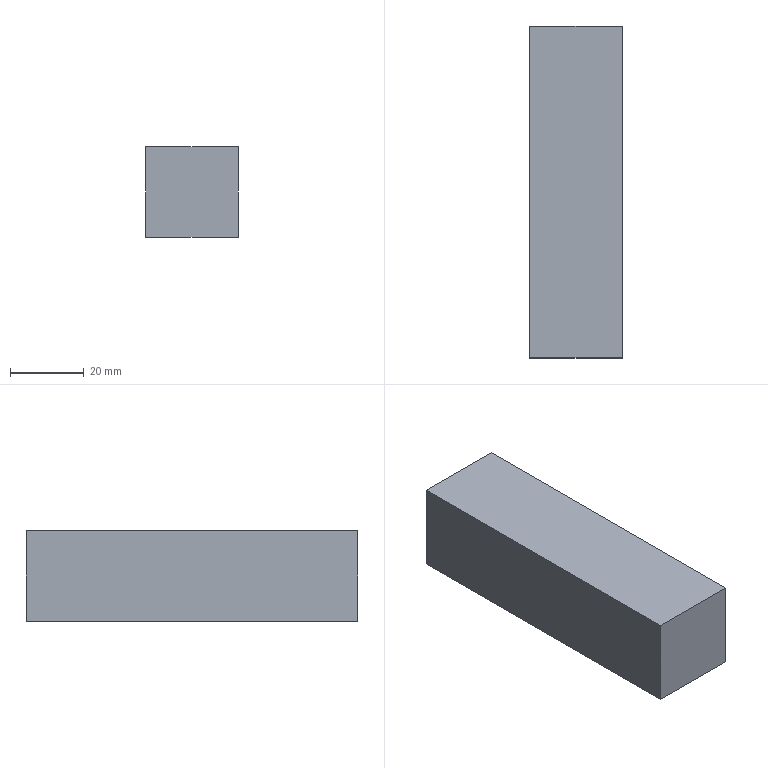Part | SolidWorks | features Extrusion 1 | 1 solid | 6 faces | box 25 x 90 x 24.5 mm | volume 55125 mm3 | plane 6
STEP:
#1=CARTESIAN_POINT('',(0.,45.,0.));
#2=VERTEX_POINT('',#1);
#3=CARTESIAN_POINT('',(0.,-45.,0.));
#4=VERTEX_POINT('',#3);
#5=CARTESIAN_POINT('',(0.,45.,0.));
#6=DIRECTION('',(0.,-1.,0.));
#7=VECTOR('',#6,1000.);
#8=LINE('',#5,#7);
#9=EDGE_CURVE('',#2,#4,#8,.T.);
#10=ORIENTED_EDGE('',*,*,#9,.T.);
#11=CARTESIAN_POINT('',(0.,-45.,24.5));
#12=VERTEX_POINT('',#11);
#13=CARTESIAN_POINT('',(0.,-45.,24.5));
#14=DIRECTION('',(0.,0.,-1.));
#15=VECTOR('',#14,1000.);
#16=LINE('',#13,#15);
#17=EDGE_CURVE('',#12,#4,#16,.T.);
#18=ORIENTED_EDGE('',*,*,#17,.F.);
#19=CARTESIAN_POINT('',(0.,45.,24.5));
#20=VERTEX_POINT('',#19);
#21=CARTESIAN_POINT('',(0.,45.,24.5));
#22=DIRECTION('',(0.,-1.,0.));
#23=VECTOR('',#22,1000.);
#24=LINE('',#21,#23);
#25=EDGE_CURVE('',#20,#12,#24,.T.);
#26=ORIENTED_EDGE('',*,*,#25,.F.);
#27=CARTESIAN_POINT('',(0.,45.,24.5));
#28=DIRECTION('',(0.,0.,-1.));
#29=VECTOR('',#28,1000.);
#30=LINE('',#27,#29);
#31=EDGE_CURVE('',#20,#2,#30,.T.);
#32=ORIENTED_EDGE('',*,*,#31,.T.);
#33=EDGE_LOOP('',(#10,#18,#26,#32));
#34=FACE_OUTER_BOUND('',#33,.T.);
#35=CARTESIAN_POINT('',(0.,45.,24.5));
#36=DIRECTION('',(1.,0.,0.));
#37=DIRECTION('',(0.,0.,-1.));
#38=AXIS2_PLACEMENT_3D('',#35,#36,#37);
#39=PLANE('',#38);
#40=ADVANCED_FACE('',(#34),#39,.F.);
#41=CARTESIAN_POINT('',(25.,-45.,0.));
#42=VERTEX_POINT('',#41);
#43=CARTESIAN_POINT('',(0.,-45.,0.));
#44=DIRECTION('',(1.,0.,0.));
#45=VECTOR('',#44,1000.);
#46=LINE('',#43,#45);
#47=EDGE_CURVE('',#4,#42,#46,.T.);
#48=ORIENTED_EDGE('',*,*,#47,.T.);
#49=CARTESIAN_POINT('',(25.,-45.,24.5));
#50=VERTEX_POINT('',#49);
#51=CARTESIAN_POINT('',(25.,-45.,24.5));
#52=DIRECTION('',(0.,0.,-1.));
#53=VECTOR('',#52,1000.);
#54=LINE('',#51,#53);
#55=EDGE_CURVE('',#50,#42,#54,.T.);
#56=ORIENTED_EDGE('',*,*,#55,.F.);
#57=CARTESIAN_POINT('',(0.,-45.,24.5));
#58=DIRECTION('',(1.,0.,0.));
#59=VECTOR('',#58,1000.);
#60=LINE('',#57,#59);
#61=EDGE_CURVE('',#12,#50,#60,.T.);
#62=ORIENTED_EDGE('',*,*,#61,.F.);
#63=ORIENTED_EDGE('',*,*,#17,.T.);
#64=EDGE_LOOP('',(#48,#56,#62,#63));
#65=FACE_OUTER_BOUND('',#64,.T.);
#66=CARTESIAN_POINT('',(0.,-45.,24.5));
#67=DIRECTION('',(0.,1.,0.));
#68=DIRECTION('',(0.,0.,1.));
#69=AXIS2_PLACEMENT_3D('',#66,#67,#68);
#70=PLANE('',#69);
#71=ADVANCED_FACE('',(#65),#70,.F.);
#72=CARTESIAN_POINT('',(25.,45.,0.));
#73=VERTEX_POINT('',#72);
#74=CARTESIAN_POINT('',(25.,45.,0.));
#75=DIRECTION('',(0.,1.,0.));
#76=VECTOR('',#75,1000.);
#77=LINE('',#74,#76);
#78=EDGE_CURVE('',#42,#73,#77,.T.);
#79=ORIENTED_EDGE('',*,*,#78,.T.);
#80=CARTESIAN_POINT('',(25.,45.,24.5));
#81=VERTEX_POINT('',#80);
#82=CARTESIAN_POINT('',(25.,45.,24.5));
#83=DIRECTION('',(0.,0.,-1.));
#84=VECTOR('',#83,1000.);
#85=LINE('',#82,#84);
#86=EDGE_CURVE('',#81,#73,#85,.T.);
#87=ORIENTED_EDGE('',*,*,#86,.F.);
#88=CARTESIAN_POINT('',(25.,45.,24.5));
#89=DIRECTION('',(0.,1.,0.));
#90=VECTOR('',#89,1000.);
#91=LINE('',#88,#90);
#92=EDGE_CURVE('',#50,#81,#91,.T.);
#93=ORIENTED_EDGE('',*,*,#92,.F.);
#94=ORIENTED_EDGE('',*,*,#55,.T.);
#95=EDGE_LOOP('',(#79,#87,#93,#94));
#96=FACE_OUTER_BOUND('',#95,.T.);
#97=CARTESIAN_POINT('',(25.,45.,24.5));
#98=DIRECTION('',(-1.,0.,0.));
#99=DIRECTION('',(0.,-1.,0.));
#100=AXIS2_PLACEMENT_3D('',#97,#98,#99);
#101=PLANE('',#100);
#102=ADVANCED_FACE('',(#96),#101,.F.);
#103=CARTESIAN_POINT('',(0.,45.,0.));
#104=DIRECTION('',(-1.,0.,0.));
#105=VECTOR('',#104,1000.);
#106=LINE('',#103,#105);
#107=EDGE_CURVE('',#73,#2,#106,.T.);
#108=ORIENTED_EDGE('',*,*,#107,.T.);
#109=ORIENTED_EDGE('',*,*,#31,.F.);
#110=CARTESIAN_POINT('',(0.,45.,24.5));
#111=DIRECTION('',(-1.,0.,0.));
#112=VECTOR('',#111,1000.);
#113=LINE('',#110,#112);
#114=EDGE_CURVE('',#81,#20,#113,.T.);
#115=ORIENTED_EDGE('',*,*,#114,.F.);
#116=ORIENTED_EDGE('',*,*,#86,.T.);
#117=EDGE_LOOP('',(#108,#109,#115,#116));
#118=FACE_OUTER_BOUND('',#117,.T.);
#119=CARTESIAN_POINT('',(0.,45.,24.5));
#120=DIRECTION('',(0.,-1.,0.));
#121=DIRECTION('',(0.,0.,-1.));
#122=AXIS2_PLACEMENT_3D('',#119,#120,#121);
#123=PLANE('',#122);
#124=ADVANCED_FACE('',(#118),#123,.F.);
#125=ORIENTED_EDGE('',*,*,#25,.T.);
#126=ORIENTED_EDGE('',*,*,#61,.T.);
#127=ORIENTED_EDGE('',*,*,#92,.T.);
#128=ORIENTED_EDGE('',*,*,#114,.T.);
#129=EDGE_LOOP('',(#125,#126,#127,#128));
#130=FACE_OUTER_BOUND('',#129,.T.);
#131=CARTESIAN_POINT('',(0.,0.,24.5));
#132=DIRECTION('',(0.,0.,1.));
#133=DIRECTION('',(1.,0.,0.));
#134=AXIS2_PLACEMENT_3D('',#131,#132,#133);
#135=PLANE('',#134);
#136=ADVANCED_FACE('',(#130),#135,.T.);
#137=ORIENTED_EDGE('',*,*,#9,.F.);
#138=ORIENTED_EDGE('',*,*,#107,.F.);
#139=ORIENTED_EDGE('',*,*,#78,.F.);
#140=ORIENTED_EDGE('',*,*,#47,.F.);
#141=EDGE_LOOP('',(#137,#138,#139,#140));
#142=FACE_OUTER_BOUND('',#141,.T.);
#143=CARTESIAN_POINT('',(0.,0.,0.));
#144=DIRECTION('',(0.,0.,1.));
#145=DIRECTION('',(1.,0.,0.));
#146=AXIS2_PLACEMENT_3D('',#143,#144,#145);
#147=PLANE('',#146);
#148=ADVANCED_FACE('',(#142),#147,.F.);
#149=CLOSED_SHELL('',(#40,#71,#102,#124,#136,#148));
#150=MANIFOLD_SOLID_BREP('',#149);
#151=CARTESIAN_POINT('',(0.,0.,0.));
#152=DIRECTION('',(0.,0.,1.));
#153=DIRECTION('',(1.,0.,0.));
#154=AXIS2_PLACEMENT_3D('',#151,#152,#153);
#155=(LENGTH_UNIT()NAMED_UNIT(*)SI_UNIT(.MILLI.,.METRE.));
#156=UNCERTAINTY_MEASURE_WITH_UNIT(LENGTH_MEASURE(0.00001),#155,'','');
#157=(NAMED_UNIT(*)PLANE_ANGLE_UNIT()SI_UNIT($,.RADIAN.));
#158=(NAMED_UNIT(*)SI_UNIT($,.STERADIAN.)SOLID_ANGLE_UNIT());
#159=(GEOMETRIC_REPRESENTATION_CONTEXT(3)GLOBAL_UNCERTAINTY_ASSIGNED_CONTEXT((#156))GLOBAL_UNIT_ASSIGNED_CONTEXT((#155,#157,#158))REPRESENTATION_CONTEXT('',''));
#160=ADVANCED_BREP_SHAPE_REPRESENTATION('',(#150,#154),#159);